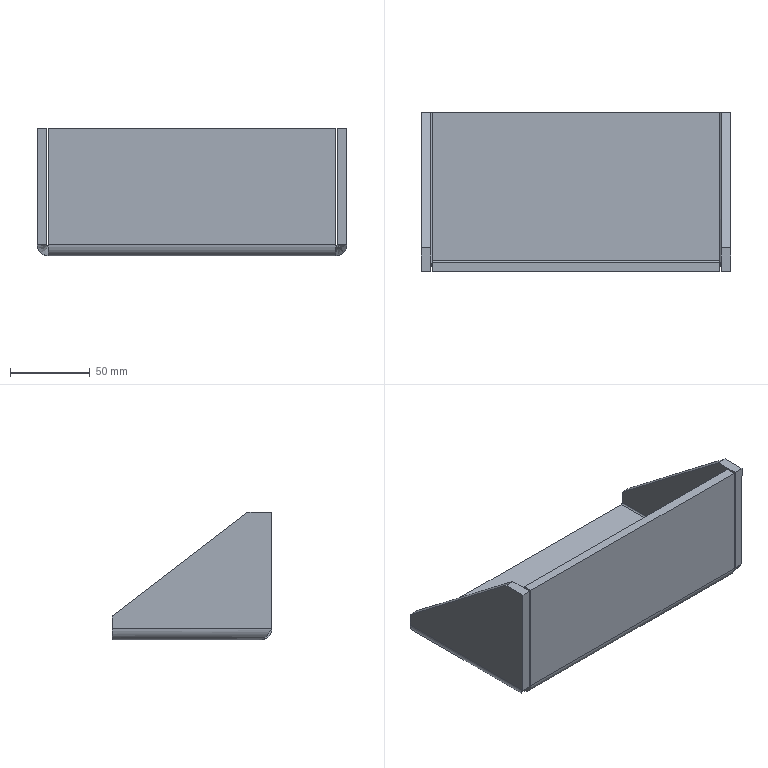Part | SolidWorks | features Chamfer 2, CornerFeat 2, EdgeFlange 2, FlatPattern 1, SMBaseFlange 1, SheetMetal 1 | 1 solid | 32 faces | box 194 x 100 x 80 mm | volume 247792 mm3 | plane 24 | cylinder 6 | spline 2 | commonest cylinder face diameters 2 x3 14 x3
STEP:
#1=CARTESIAN_POINT('',(-90.,1.,-40.));
#2=VERTEX_POINT('',#1);
#3=CARTESIAN_POINT('',(90.,1.,-40.));
#4=VERTEX_POINT('',#3);
#5=CARTESIAN_POINT('',(90.,1.,-40.));
#6=DIRECTION('',(1.,0.,0.));
#7=VECTOR('',#6,1000.);
#8=LINE('',#5,#7);
#9=EDGE_CURVE('',#2,#4,#8,.T.);
#10=ORIENTED_EDGE('',*,*,#9,.F.);
#11=CARTESIAN_POINT('',(-90.,94.,-40.));
#12=VERTEX_POINT('',#11);
#13=CARTESIAN_POINT('',(-90.,0.,-40.));
#14=DIRECTION('',(0.,1.,0.));
#15=VECTOR('',#14,1000.);
#16=LINE('',#13,#15);
#17=EDGE_CURVE('',#2,#12,#16,.T.);
#18=ORIENTED_EDGE('',*,*,#17,.T.);
#19=CARTESIAN_POINT('',(90.,94.,-40.));
#20=VERTEX_POINT('',#19);
#21=CARTESIAN_POINT('',(0.,94.,-40.));
#22=DIRECTION('',(1.,0.,0.));
#23=VECTOR('',#22,1000.);
#24=LINE('',#21,#23);
#25=EDGE_CURVE('',#12,#20,#24,.T.);
#26=ORIENTED_EDGE('',*,*,#25,.T.);
#27=CARTESIAN_POINT('',(90.,0.,-40.));
#28=DIRECTION('',(0.,-1.,0.));
#29=VECTOR('',#28,1000.);
#30=LINE('',#27,#29);
#31=EDGE_CURVE('',#20,#4,#30,.T.);
#32=ORIENTED_EDGE('',*,*,#31,.T.);
#33=EDGE_LOOP('',(#10,#18,#26,#32));
#34=FACE_OUTER_BOUND('',#33,.T.);
#35=CARTESIAN_POINT('',(0.,0.,-40.));
#36=DIRECTION('',(0.,0.,1.));
#37=DIRECTION('',(0.,-1.,0.));
#38=AXIS2_PLACEMENT_3D('',#35,#36,#37);
#39=PLANE('',#38);
#40=ADVANCED_FACE('',(#34),#39,.F.);
#41=CARTESIAN_POINT('',(-90.,1.,-34.));
#42=VERTEX_POINT('',#41);
#43=CARTESIAN_POINT('',(-90.,94.,-34.));
#44=VERTEX_POINT('',#43);
#45=CARTESIAN_POINT('',(-90.,94.,-34.));
#46=DIRECTION('',(0.,1.,0.));
#47=VECTOR('',#46,1000.);
#48=LINE('',#45,#47);
#49=EDGE_CURVE('',#42,#44,#48,.T.);
#50=ORIENTED_EDGE('',*,*,#49,.F.);
#51=CARTESIAN_POINT('',(90.,1.,-34.));
#52=VERTEX_POINT('',#51);
#53=CARTESIAN_POINT('',(90.,1.,-34.));
#54=DIRECTION('',(-1.,0.,0.));
#55=VECTOR('',#54,1000.);
#56=LINE('',#53,#55);
#57=EDGE_CURVE('',#52,#42,#56,.T.);
#58=ORIENTED_EDGE('',*,*,#57,.F.);
#59=CARTESIAN_POINT('',(90.,94.,-34.));
#60=VERTEX_POINT('',#59);
#61=CARTESIAN_POINT('',(90.,0.,-34.));
#62=DIRECTION('',(0.,-1.,0.));
#63=VECTOR('',#62,1000.);
#64=LINE('',#61,#63);
#65=EDGE_CURVE('',#60,#52,#64,.T.);
#66=ORIENTED_EDGE('',*,*,#65,.F.);
#67=CARTESIAN_POINT('',(90.,94.,-34.));
#68=DIRECTION('',(1.,0.,0.));
#69=VECTOR('',#68,1000.);
#70=LINE('',#67,#69);
#71=EDGE_CURVE('',#44,#60,#70,.T.);
#72=ORIENTED_EDGE('',*,*,#71,.F.);
#73=EDGE_LOOP('',(#50,#58,#66,#72));
#74=FACE_OUTER_BOUND('',#73,.T.);
#75=CARTESIAN_POINT('',(0.,0.,-34.));
#76=DIRECTION('',(0.,0.,1.));
#77=DIRECTION('',(0.,-1.,0.));
#78=AXIS2_PLACEMENT_3D('',#75,#76,#77);
#79=PLANE('',#78);
#80=ADVANCED_FACE('',(#74),#79,.T.);
#81=ORIENTED_EDGE('',*,*,#71,.T.);
#82=CARTESIAN_POINT('',(90.,94.,-40.));
#83=DIRECTION('',(0.,0.,1.));
#84=VECTOR('',#83,1000.);
#85=LINE('',#82,#84);
#86=EDGE_CURVE('',#20,#60,#85,.T.);
#87=ORIENTED_EDGE('',*,*,#86,.F.);
#88=ORIENTED_EDGE('',*,*,#25,.F.);
#89=CARTESIAN_POINT('',(-90.,94.,-40.));
#90=DIRECTION('',(0.,0.,1.));
#91=VECTOR('',#90,1000.);
#92=LINE('',#89,#91);
#93=EDGE_CURVE('',#12,#44,#92,.T.);
#94=ORIENTED_EDGE('',*,*,#93,.T.);
#95=EDGE_LOOP('',(#81,#87,#88,#94));
#96=FACE_OUTER_BOUND('',#95,.T.);
#97=CARTESIAN_POINT('',(90.,94.,-40.));
#98=DIRECTION('',(0.,-1.,0.));
#99=DIRECTION('',(0.,0.,-1.));
#100=AXIS2_PLACEMENT_3D('',#97,#98,#99);
#101=PLANE('',#100);
#102=ADVANCED_FACE('',(#96),#101,.F.);
#103=CARTESIAN_POINT('',(-97.,9.,40.));
#104=VERTEX_POINT('',#103);
#105=CARTESIAN_POINT('',(-97.,94.,-25.));
#106=VERTEX_POINT('',#105);
#107=CARTESIAN_POINT('',(-97.,94.,-25.));
#108=DIRECTION('',(0.,0.7944,-0.6075));
#109=VECTOR('',#108,1000.);
#110=LINE('',#107,#109);
#111=EDGE_CURVE('',#104,#106,#110,.T.);
#112=ORIENTED_EDGE('',*,*,#111,.F.);
#113=CARTESIAN_POINT('',(-91.,9.,40.));
#114=VERTEX_POINT('',#113);
#115=CARTESIAN_POINT('',(-97.,9.,40.));
#116=DIRECTION('',(-1.,0.,0.));
#117=VECTOR('',#116,1000.);
#118=LINE('',#115,#117);
#119=EDGE_CURVE('',#114,#104,#118,.T.);
#120=ORIENTED_EDGE('',*,*,#119,.F.);
#121=CARTESIAN_POINT('',(-91.,94.,-25.));
#122=VERTEX_POINT('',#121);
#123=CARTESIAN_POINT('',(-91.,22.622,29.583));
#124=DIRECTION('',(0.,-0.7944,0.6075));
#125=VECTOR('',#124,1000.);
#126=LINE('',#123,#125);
#127=EDGE_CURVE('',#122,#114,#126,.T.);
#128=ORIENTED_EDGE('',*,*,#127,.F.);
#129=CARTESIAN_POINT('',(-97.,94.,-25.));
#130=DIRECTION('',(1.,0.,0.));
#131=VECTOR('',#130,1000.);
#132=LINE('',#129,#131);
#133=EDGE_CURVE('',#106,#122,#132,.T.);
#134=ORIENTED_EDGE('',*,*,#133,.F.);
#135=EDGE_LOOP('',(#112,#120,#128,#134));
#136=FACE_OUTER_BOUND('',#135,.T.);
#137=CARTESIAN_POINT('',(-97.,94.,-25.));
#138=DIRECTION('',(0.,-0.6075,-0.7944));
#139=DIRECTION('',(1.,0.,0.));
#140=AXIS2_PLACEMENT_3D('',#137,#138,#139);
#141=PLANE('',#140);
#142=ADVANCED_FACE('',(#136),#141,.F.);
#143=CARTESIAN_POINT('',(-91.,-6.,40.));
#144=VERTEX_POINT('',#143);
#145=CARTESIAN_POINT('',(-91.,94.,40.));
#146=DIRECTION('',(0.,1.,0.));
#147=VECTOR('',#146,1000.);
#148=LINE('',#145,#147);
#149=EDGE_CURVE('',#144,#114,#148,.T.);
#150=ORIENTED_EDGE('',*,*,#149,.T.);
#151=ORIENTED_EDGE('',*,*,#119,.T.);
#152=CARTESIAN_POINT('',(-97.,-6.,40.));
#153=VERTEX_POINT('',#152);
#154=CARTESIAN_POINT('',(-97.,0.,40.));
#155=DIRECTION('',(0.,1.,0.));
#156=VECTOR('',#155,1000.);
#157=LINE('',#154,#156);
#158=EDGE_CURVE('',#153,#104,#157,.T.);
#159=ORIENTED_EDGE('',*,*,#158,.F.);
#160=CARTESIAN_POINT('',(-97.,-6.,40.));
#161=DIRECTION('',(1.,0.,0.));
#162=VECTOR('',#161,1000.);
#163=LINE('',#160,#162);
#164=EDGE_CURVE('',#153,#144,#163,.T.);
#165=ORIENTED_EDGE('',*,*,#164,.T.);
#166=EDGE_LOOP('',(#150,#151,#159,#165));
#167=FACE_OUTER_BOUND('',#166,.T.);
#168=CARTESIAN_POINT('',(-97.,94.,40.));
#169=DIRECTION('',(0.,0.,-1.));
#170=DIRECTION('',(-1.,0.,0.));
#171=AXIS2_PLACEMENT_3D('',#168,#169,#170);
#172=PLANE('',#171);
#173=ADVANCED_FACE('',(#167),#172,.F.);
#174=ORIENTED_EDGE('',*,*,#158,.T.);
#175=ORIENTED_EDGE('',*,*,#111,.T.);
#176=CARTESIAN_POINT('',(-97.,94.,-33.));
#177=VERTEX_POINT('',#176);
#178=CARTESIAN_POINT('',(-97.,94.,0.));
#179=DIRECTION('',(0.,0.,-1.));
#180=VECTOR('',#179,1000.);
#181=LINE('',#178,#180);
#182=EDGE_CURVE('',#106,#177,#181,.T.);
#183=ORIENTED_EDGE('',*,*,#182,.T.);
#184=CARTESIAN_POINT('',(-97.,-6.,-33.));
#185=VERTEX_POINT('',#184);
#186=CARTESIAN_POINT('',(-97.,94.,-33.));
#187=DIRECTION('',(0.,1.,0.));
#188=VECTOR('',#187,1000.);
#189=LINE('',#186,#188);
#190=EDGE_CURVE('',#185,#177,#189,.T.);
#191=ORIENTED_EDGE('',*,*,#190,.F.);
#192=CARTESIAN_POINT('',(-97.,-6.,-33.));
#193=DIRECTION('',(0.,0.,1.));
#194=VECTOR('',#193,1000.);
#195=LINE('',#192,#194);
#196=EDGE_CURVE('',#185,#153,#195,.T.);
#197=ORIENTED_EDGE('',*,*,#196,.T.);
#198=EDGE_LOOP('',(#174,#175,#183,#191,#197));
#199=FACE_OUTER_BOUND('',#198,.T.);
#200=CARTESIAN_POINT('',(-97.,0.,0.));
#201=DIRECTION('',(1.,0.,0.));
#202=DIRECTION('',(0.,0.,-1.));
#203=AXIS2_PLACEMENT_3D('',#200,#201,#202);
#204=PLANE('',#203);
#205=ADVANCED_FACE('',(#199),#204,.F.);
#206=CARTESIAN_POINT('',(-91.,-6.,-33.));
#207=VERTEX_POINT('',#206);
#208=CARTESIAN_POINT('',(-91.,-6.,-33.));
#209=DIRECTION('',(0.,0.,1.));
#210=VECTOR('',#209,1000.);
#211=LINE('',#208,#210);
#212=EDGE_CURVE('',#207,#144,#211,.T.);
#213=ORIENTED_EDGE('',*,*,#212,.T.);
#214=ORIENTED_EDGE('',*,*,#164,.F.);
#215=ORIENTED_EDGE('',*,*,#196,.F.);
#216=CARTESIAN_POINT('',(-97.,-6.,-33.));
#217=CARTESIAN_POINT('',(-95.,-6.,-33.));
#218=CARTESIAN_POINT('',(-93.,-6.,-33.));
#219=CARTESIAN_POINT('',(-91.,-6.,-33.));
#220=B_SPLINE_CURVE_WITH_KNOTS('',3,(#216,#217,#218,#219),.UNSPECIFIED.,.F.,.F.,(4,4),(0.,1.),.UNSPECIFIED.);
#221=EDGE_CURVE('',#185,#207,#220,.T.);
#222=ORIENTED_EDGE('',*,*,#221,.T.);
#223=EDGE_LOOP('',(#213,#214,#215,#222));
#224=FACE_OUTER_BOUND('',#223,.T.);
#225=CARTESIAN_POINT('',(-97.,-6.,-33.));
#226=DIRECTION('',(0.,1.,0.));
#227=DIRECTION('',(-1.,0.,0.));
#228=AXIS2_PLACEMENT_3D('',#225,#226,#227);
#229=PLANE('',#228);
#230=ADVANCED_FACE('',(#224),#229,.F.);
#231=CARTESIAN_POINT('',(-91.,94.,-33.));
#232=VERTEX_POINT('',#231);
#233=CARTESIAN_POINT('',(-91.,94.,-34.));
#234=DIRECTION('',(0.,0.,-1.));
#235=VECTOR('',#234,1000.);
#236=LINE('',#233,#235);
#237=EDGE_CURVE('',#122,#232,#236,.T.);
#238=ORIENTED_EDGE('',*,*,#237,.F.);
#239=ORIENTED_EDGE('',*,*,#127,.T.);
#240=ORIENTED_EDGE('',*,*,#149,.F.);
#241=ORIENTED_EDGE('',*,*,#212,.F.);
#242=CARTESIAN_POINT('',(-91.,94.,-33.));
#243=DIRECTION('',(0.,-1.,0.));
#244=VECTOR('',#243,1000.);
#245=LINE('',#242,#244);
#246=EDGE_CURVE('',#232,#207,#245,.T.);
#247=ORIENTED_EDGE('',*,*,#246,.F.);
#248=EDGE_LOOP('',(#238,#239,#240,#241,#247));
#249=FACE_OUTER_BOUND('',#248,.T.);
#250=CARTESIAN_POINT('',(-91.,0.,0.));
#251=DIRECTION('',(1.,0.,0.));
#252=DIRECTION('',(0.,0.,-1.));
#253=AXIS2_PLACEMENT_3D('',#250,#251,#252);
#254=PLANE('',#253);
#255=ADVANCED_FACE('',(#249),#254,.T.);
#256=ORIENTED_EDGE('',*,*,#182,.F.);
#257=ORIENTED_EDGE('',*,*,#133,.T.);
#258=ORIENTED_EDGE('',*,*,#237,.T.);
#259=CARTESIAN_POINT('',(-97.,94.,-33.));
#260=DIRECTION('',(-1.,0.,0.));
#261=VECTOR('',#260,1000.);
#262=LINE('',#259,#261);
#263=EDGE_CURVE('',#232,#177,#262,.T.);
#264=ORIENTED_EDGE('',*,*,#263,.T.);
#265=EDGE_LOOP('',(#256,#257,#258,#264));
#266=FACE_OUTER_BOUND('',#265,.T.);
#267=CARTESIAN_POINT('',(-97.,94.,-34.));
#268=DIRECTION('',(0.,-1.,0.));
#269=DIRECTION('',(0.,0.,-1.));
#270=AXIS2_PLACEMENT_3D('',#267,#268,#269);
#271=PLANE('',#270);
#272=ADVANCED_FACE('',(#266),#271,.F.);
#273=ORIENTED_EDGE('',*,*,#263,.F.);
#274=CARTESIAN_POINT('',(-90.,94.,-33.));
#275=DIRECTION('',(0.,-1.,0.));
#276=DIRECTION('',(0.,0.,-1.));
#277=AXIS2_PLACEMENT_3D('',#274,#275,#276);
#278=CIRCLE('',#277,1.);
#279=EDGE_CURVE('',#232,#44,#278,.T.);
#280=ORIENTED_EDGE('',*,*,#279,.T.);
#281=ORIENTED_EDGE('',*,*,#93,.F.);
#282=CARTESIAN_POINT('',(-90.,94.,-33.));
#283=DIRECTION('',(0.,-1.,0.));
#284=DIRECTION('',(0.,0.,-1.));
#285=AXIS2_PLACEMENT_3D('',#282,#283,#284);
#286=CIRCLE('',#285,7.);
#287=EDGE_CURVE('',#177,#12,#286,.T.);
#288=ORIENTED_EDGE('',*,*,#287,.F.);
#289=EDGE_LOOP('',(#273,#280,#281,#288));
#290=FACE_OUTER_BOUND('',#289,.T.);
#291=CARTESIAN_POINT('',(-90.,94.,-33.));
#292=DIRECTION('',(0.,1.,0.));
#293=DIRECTION('',(0.,0.,1.));
#294=AXIS2_PLACEMENT_3D('',#291,#292,#293);
#295=PLANE('',#294);
#296=ADVANCED_FACE('',(#290),#295,.T.);
#297=CARTESIAN_POINT('',(-90.,1.,-34.));
#298=CARTESIAN_POINT('',(-90.131,0.4159,-34.));
#299=CARTESIAN_POINT('',(-90.262,-0.1669,-33.974));
#300=CARTESIAN_POINT('',(-90.504,-1.335,-33.874));
#301=CARTESIAN_POINT('',(-90.615,-1.918,-33.799));
#302=CARTESIAN_POINT('',(-90.8,-3.085,-33.614));
#303=CARTESIAN_POINT('',(-90.874,-3.669,-33.503));
#304=CARTESIAN_POINT('',(-90.974,-4.834,-33.262));
#305=CARTESIAN_POINT('',(-91.,-5.416,-33.131));
#306=CARTESIAN_POINT('',(-91.,-6.,-33.));
#307=B_SPLINE_CURVE_WITH_KNOTS('',3,(#297,#298,#299,#300,#301,#302,#303,#304,#305,#306),.UNSPECIFIED.,.F.,.F.,(4,2,2,2,4),(0.,0.001794,0.003587,0.005381,0.007175),.UNSPECIFIED.);
#308=EDGE_CURVE('',#42,#207,#307,.T.);
#309=ORIENTED_EDGE('',*,*,#308,.T.);
#310=ORIENTED_EDGE('',*,*,#221,.F.);
#311=CARTESIAN_POINT('',(-90.,1.,-40.));
#312=CARTESIAN_POINT('',(-90.462,0.7056,-40.));
#313=CARTESIAN_POINT('',(-90.919,0.4151,-39.954));
#314=CARTESIAN_POINT('',(-91.814,-0.1663,-39.776));
#315=CARTESIAN_POINT('',(-92.256,-0.4585,-39.643));
#316=CARTESIAN_POINT('',(-93.108,-1.046,-39.289));
#317=CARTESIAN_POINT('',(-93.511,-1.336,-39.073));
#318=CARTESIAN_POINT('',(-94.269,-1.916,-38.566));
#319=CARTESIAN_POINT('',(-94.625,-2.207,-38.275));
#320=CARTESIAN_POINT('',(-95.604,-3.089,-37.295));
#321=CARTESIAN_POINT('',(-96.114,-3.662,-36.532));
#322=CARTESIAN_POINT('',(-96.821,-4.839,-34.824));
#323=CARTESIAN_POINT('',(-97.,-5.411,-33.925));
#324=CARTESIAN_POINT('',(-97.,-6.,-33.));
#325=B_SPLINE_CURVE_WITH_KNOTS('',3,(#311,#312,#313,#314,#315,#316,#317,#318,#319,#320,#321,#322,#323,#324),.UNSPECIFIED.,.F.,.F.,(4,2,2,2,2,2,4),(0.,0.001624,0.003248,0.004872,0.006496,0.009744,0.01299),.UNSPECIFIED.);
#326=EDGE_CURVE('',#2,#185,#325,.T.);
#327=ORIENTED_EDGE('',*,*,#326,.F.);
#328=CARTESIAN_POINT('',(-90.,1.,-34.));
#329=CARTESIAN_POINT('',(-90.,1.,-36.));
#330=CARTESIAN_POINT('',(-90.,1.,-38.));
#331=CARTESIAN_POINT('',(-90.,1.,-40.));
#332=B_SPLINE_CURVE_WITH_KNOTS('',3,(#328,#329,#330,#331),.UNSPECIFIED.,.F.,.F.,(4,4),(0.,1.),.UNSPECIFIED.);
#333=EDGE_CURVE('',#42,#2,#332,.T.);
#334=ORIENTED_EDGE('',*,*,#333,.F.);
#335=EDGE_LOOP('',(#309,#310,#327,#334));
#336=FACE_OUTER_BOUND('',#335,.T.);
#337=CARTESIAN_POINT('',(-90.,1.,-40.061));
#338=CARTESIAN_POINT('',(-90.924,0.4166,-40.061));
#339=CARTESIAN_POINT('',(-91.848,-0.1667,-39.877));
#340=CARTESIAN_POINT('',(-93.556,-1.333,-39.169));
#341=CARTESIAN_POINT('',(-94.339,-1.917,-38.646));
#342=CARTESIAN_POINT('',(-95.646,-3.083,-37.339));
#343=CARTESIAN_POINT('',(-96.169,-3.667,-36.556));
#344=CARTESIAN_POINT('',(-96.877,-4.833,-34.848));
#345=CARTESIAN_POINT('',(-97.061,-5.417,-33.924));
#346=CARTESIAN_POINT('',(-97.061,-6.,-33.));
#347=CARTESIAN_POINT('',(-90.,1.,-40.));
#348=CARTESIAN_POINT('',(-90.916,0.4166,-40.));
#349=CARTESIAN_POINT('',(-91.832,-0.1667,-39.818));
#350=CARTESIAN_POINT('',(-93.525,-1.333,-39.117));
#351=CARTESIAN_POINT('',(-94.302,-1.917,-38.598));
#352=CARTESIAN_POINT('',(-95.598,-3.083,-37.302));
#353=CARTESIAN_POINT('',(-96.117,-3.667,-36.525));
#354=CARTESIAN_POINT('',(-96.818,-4.833,-34.832));
#355=CARTESIAN_POINT('',(-97.,-5.417,-33.916));
#356=CARTESIAN_POINT('',(-97.,-6.,-33.));
#357=CARTESIAN_POINT('',(-90.,1.,-34.));
#358=CARTESIAN_POINT('',(-90.131,0.4167,-34.));
#359=CARTESIAN_POINT('',(-90.262,-0.1667,-33.974));
#360=CARTESIAN_POINT('',(-90.504,-1.333,-33.874));
#361=CARTESIAN_POINT('',(-90.615,-1.917,-33.8));
#362=CARTESIAN_POINT('',(-90.8,-3.083,-33.615));
#363=CARTESIAN_POINT('',(-90.874,-3.667,-33.504));
#364=CARTESIAN_POINT('',(-90.974,-4.833,-33.262));
#365=CARTESIAN_POINT('',(-91.,-5.417,-33.131));
#366=CARTESIAN_POINT('',(-91.,-6.,-33.));
#367=CARTESIAN_POINT('',(-90.,1.,-33.94));
#368=CARTESIAN_POINT('',(-90.123,0.4167,-33.94));
#369=CARTESIAN_POINT('',(-90.246,-0.1667,-33.916));
#370=CARTESIAN_POINT('',(-90.473,-1.333,-33.821));
#371=CARTESIAN_POINT('',(-90.578,-1.917,-33.752));
#372=CARTESIAN_POINT('',(-90.752,-3.083,-33.578));
#373=CARTESIAN_POINT('',(-90.821,-3.667,-33.473));
#374=CARTESIAN_POINT('',(-90.916,-4.833,-33.246));
#375=CARTESIAN_POINT('',(-90.94,-5.417,-33.123));
#376=CARTESIAN_POINT('',(-90.94,-6.,-33.));
#377=B_SPLINE_SURFACE_WITH_KNOTS('',1,3,((#337,#338,#339,#340,#341,#342,#343,#344,#345,#346),(#347,#348,#349,#350,#351,#352,#353,#354,#355,#356),(#357,#358,#359,#360,#361,#362,#363,#364,#365,#366),(#367,#368,#369,#370,#371,#372,#373,#374,#375,#376)),.UNSPECIFIED.,.F.,.F.,.F.,(2,1,1,2),(4,2,2,2,4),(-0.0101,0.,1.,1.01),(0.,0.25,0.5,0.75,1.),.UNSPECIFIED.);
#378=ADVANCED_FACE('',(#336),#377,.T.);
#379=ORIENTED_EDGE('',*,*,#17,.F.);
#380=ORIENTED_EDGE('',*,*,#326,.T.);
#381=ORIENTED_EDGE('',*,*,#190,.T.);
#382=ORIENTED_EDGE('',*,*,#287,.T.);
#383=EDGE_LOOP('',(#379,#380,#381,#382));
#384=FACE_OUTER_BOUND('',#383,.T.);
#385=CARTESIAN_POINT('',(-90.,144.377,-33.));
#386=DIRECTION('',(0.,-1.,0.));
#387=DIRECTION('',(0.,0.,-1.));
#388=AXIS2_PLACEMENT_3D('',#385,#386,#387);
#389=CYLINDRICAL_SURFACE('',#388,7.);
#390=ADVANCED_FACE('',(#384),#389,.T.);
#391=ORIENTED_EDGE('',*,*,#49,.T.);
#392=ORIENTED_EDGE('',*,*,#279,.F.);
#393=ORIENTED_EDGE('',*,*,#246,.T.);
#394=ORIENTED_EDGE('',*,*,#308,.F.);
#395=EDGE_LOOP('',(#391,#392,#393,#394));
#396=FACE_OUTER_BOUND('',#395,.T.);
#397=CARTESIAN_POINT('',(-90.,144.377,-33.));
#398=DIRECTION('',(0.,-1.,0.));
#399=DIRECTION('',(0.,0.,-1.));
#400=AXIS2_PLACEMENT_3D('',#397,#398,#399);
#401=CYLINDRICAL_SURFACE('',#400,1.);
#402=ADVANCED_FACE('',(#396),#401,.F.);
#403=CARTESIAN_POINT('',(97.,9.,40.));
#404=VERTEX_POINT('',#403);
#405=CARTESIAN_POINT('',(97.,-6.,40.));
#406=VERTEX_POINT('',#405);
#407=CARTESIAN_POINT('',(97.,0.,40.));
#408=DIRECTION('',(0.,-1.,0.));
#409=VECTOR('',#408,1000.);
#410=LINE('',#407,#409);
#411=EDGE_CURVE('',#404,#406,#410,.T.);
#412=ORIENTED_EDGE('',*,*,#411,.F.);
#413=CARTESIAN_POINT('',(91.,9.,40.));
#414=VERTEX_POINT('',#413);
#415=CARTESIAN_POINT('',(97.,9.,40.));
#416=DIRECTION('',(-1.,0.,0.));
#417=VECTOR('',#416,1000.);
#418=LINE('',#415,#417);
#419=EDGE_CURVE('',#404,#414,#418,.T.);
#420=ORIENTED_EDGE('',*,*,#419,.T.);
#421=CARTESIAN_POINT('',(91.,-6.,40.));
#422=VERTEX_POINT('',#421);
#423=CARTESIAN_POINT('',(91.,1.,40.));
#424=DIRECTION('',(0.,-1.,0.));
#425=VECTOR('',#424,1000.);
#426=LINE('',#423,#425);
#427=EDGE_CURVE('',#414,#422,#426,.T.);
#428=ORIENTED_EDGE('',*,*,#427,.T.);
#429=CARTESIAN_POINT('',(97.,-6.,40.));
#430=DIRECTION('',(-1.,0.,0.));
#431=VECTOR('',#430,1000.);
#432=LINE('',#429,#431);
#433=EDGE_CURVE('',#406,#422,#432,.T.);
#434=ORIENTED_EDGE('',*,*,#433,.F.);
#435=EDGE_LOOP('',(#412,#420,#428,#434));
#436=FACE_OUTER_BOUND('',#435,.T.);
#437=CARTESIAN_POINT('',(97.,1.,40.));
#438=DIRECTION('',(0.,0.,-1.));
#439=DIRECTION('',(-1.,0.,0.));
#440=AXIS2_PLACEMENT_3D('',#437,#438,#439);
#441=PLANE('',#440);
#442=ADVANCED_FACE('',(#436),#441,.F.);
#443=CARTESIAN_POINT('',(97.,94.,-25.));
#444=VERTEX_POINT('',#443);
#445=CARTESIAN_POINT('',(97.,9.,40.));
#446=DIRECTION('',(0.,-0.7944,0.6075));
#447=VECTOR('',#446,1000.);
#448=LINE('',#445,#447);
#449=EDGE_CURVE('',#444,#404,#448,.T.);
#450=ORIENTED_EDGE('',*,*,#449,.F.);
#451=CARTESIAN_POINT('',(91.,94.,-25.));
#452=VERTEX_POINT('',#451);
#453=CARTESIAN_POINT('',(97.,94.,-25.));
#454=DIRECTION('',(1.,0.,0.));
#455=VECTOR('',#454,1000.);
#456=LINE('',#453,#455);
#457=EDGE_CURVE('',#452,#444,#456,.T.);
#458=ORIENTED_EDGE('',*,*,#457,.F.);
#459=CARTESIAN_POINT('',(91.,22.622,29.583));
#460=DIRECTION('',(0.,0.7944,-0.6075));
#461=VECTOR('',#460,1000.);
#462=LINE('',#459,#461);
#463=EDGE_CURVE('',#414,#452,#462,.T.);
#464=ORIENTED_EDGE('',*,*,#463,.F.);
#465=ORIENTED_EDGE('',*,*,#419,.F.);
#466=EDGE_LOOP('',(#450,#458,#464,#465));
#467=FACE_OUTER_BOUND('',#466,.T.);
#468=CARTESIAN_POINT('',(97.,9.,40.));
#469=DIRECTION('',(0.,-0.6075,-0.7944));
#470=DIRECTION('',(-1.,0.,0.));
#471=AXIS2_PLACEMENT_3D('',#468,#469,#470);
#472=PLANE('',#471);
#473=ADVANCED_FACE('',(#467),#472,.F.);
#474=CARTESIAN_POINT('',(97.,94.,-33.));
#475=VERTEX_POINT('',#474);
#476=CARTESIAN_POINT('',(97.,94.,0.));
#477=DIRECTION('',(0.,0.,1.));
#478=VECTOR('',#477,1000.);
#479=LINE('',#476,#478);
#480=EDGE_CURVE('',#475,#444,#479,.T.);
#481=ORIENTED_EDGE('',*,*,#480,.T.);
#482=ORIENTED_EDGE('',*,*,#449,.T.);
#483=ORIENTED_EDGE('',*,*,#411,.T.);
#484=CARTESIAN_POINT('',(97.,-6.,-33.));
#485=VERTEX_POINT('',#484);
#486=CARTESIAN_POINT('',(97.,-6.,-33.));
#487=DIRECTION('',(0.,0.,1.));
#488=VECTOR('',#487,1000.);
#489=LINE('',#486,#488);
#490=EDGE_CURVE('',#485,#406,#489,.T.);
#491=ORIENTED_EDGE('',*,*,#490,.F.);
#492=CARTESIAN_POINT('',(97.,1.,-33.));
#493=DIRECTION('',(0.,-1.,0.));
#494=VECTOR('',#493,1000.);
#495=LINE('',#492,#494);
#496=EDGE_CURVE('',#475,#485,#495,.T.);
#497=ORIENTED_EDGE('',*,*,#496,.F.);
#498=EDGE_LOOP('',(#481,#482,#483,#491,#497));
#499=FACE_OUTER_BOUND('',#498,.T.);
#500=CARTESIAN_POINT('',(97.,0.,0.));
#501=DIRECTION('',(-1.,0.,0.));
#502=DIRECTION('',(0.,0.,1.));
#503=AXIS2_PLACEMENT_3D('',#500,#501,#502);
#504=PLANE('',#503);
#505=ADVANCED_FACE('',(#499),#504,.F.);
#506=CARTESIAN_POINT('',(91.,94.,-33.));
#507=VERTEX_POINT('',#506);
#508=CARTESIAN_POINT('',(91.,94.,40.));
#509=DIRECTION('',(0.,0.,1.));
#510=VECTOR('',#509,1000.);
#511=LINE('',#508,#510);
#512=EDGE_CURVE('',#507,#452,#511,.T.);
#513=ORIENTED_EDGE('',*,*,#512,.T.);
#514=ORIENTED_EDGE('',*,*,#457,.T.);
#515=ORIENTED_EDGE('',*,*,#480,.F.);
#516=CARTESIAN_POINT('',(91.,94.,-33.));
#517=DIRECTION('',(1.,0.,0.));
#518=VECTOR('',#517,1000.);
#519=LINE('',#516,#518);
#520=EDGE_CURVE('',#507,#475,#519,.T.);
#521=ORIENTED_EDGE('',*,*,#520,.F.);
#522=EDGE_LOOP('',(#513,#514,#515,#521));
#523=FACE_OUTER_BOUND('',#522,.T.);
#524=CARTESIAN_POINT('',(97.,94.,40.));
#525=DIRECTION('',(0.,-1.,0.));
#526=DIRECTION('',(0.,0.,-1.));
#527=AXIS2_PLACEMENT_3D('',#524,#525,#526);
#528=PLANE('',#527);
#529=ADVANCED_FACE('',(#523),#528,.F.);
#530=ORIENTED_EDGE('',*,*,#427,.F.);
#531=ORIENTED_EDGE('',*,*,#463,.T.);
#532=ORIENTED_EDGE('',*,*,#512,.F.);
#533=CARTESIAN_POINT('',(91.,-6.,-33.));
#534=VERTEX_POINT('',#533);
#535=CARTESIAN_POINT('',(91.,1.,-33.));
#536=DIRECTION('',(0.,1.,0.));
#537=VECTOR('',#536,1000.);
#538=LINE('',#535,#537);
#539=EDGE_CURVE('',#534,#507,#538,.T.);
#540=ORIENTED_EDGE('',*,*,#539,.F.);
#541=CARTESIAN_POINT('',(91.,-6.,-33.));
#542=DIRECTION('',(0.,0.,1.));
#543=VECTOR('',#542,1000.);
#544=LINE('',#541,#543);
#545=EDGE_CURVE('',#534,#422,#544,.T.);
#546=ORIENTED_EDGE('',*,*,#545,.T.);
#547=EDGE_LOOP('',(#530,#531,#532,#540,#546));
#548=FACE_OUTER_BOUND('',#547,.T.);
#549=CARTESIAN_POINT('',(91.,0.,0.));
#550=DIRECTION('',(-1.,0.,0.));
#551=DIRECTION('',(0.,0.,1.));
#552=AXIS2_PLACEMENT_3D('',#549,#550,#551);
#553=PLANE('',#552);
#554=ADVANCED_FACE('',(#548),#553,.T.);
#555=ORIENTED_EDGE('',*,*,#545,.F.);
#556=CARTESIAN_POINT('',(97.,-6.,-33.));
#557=CARTESIAN_POINT('',(91.,-6.,-33.));
#558=B_SPLINE_CURVE_WITH_KNOTS('',1,(#556,#557),.UNSPECIFIED.,.F.,.F.,(2,2),(0.,1.),.UNSPECIFIED.);
#559=EDGE_CURVE('',#485,#534,#558,.T.);
#560=ORIENTED_EDGE('',*,*,#559,.F.);
#561=ORIENTED_EDGE('',*,*,#490,.T.);
#562=ORIENTED_EDGE('',*,*,#433,.T.);
#563=EDGE_LOOP('',(#555,#560,#561,#562));
#564=FACE_OUTER_BOUND('',#563,.T.);
#565=CARTESIAN_POINT('',(97.,-6.,-33.));
#566=DIRECTION('',(0.,-1.,0.));
#567=DIRECTION('',(1.,0.,0.));
#568=AXIS2_PLACEMENT_3D('',#565,#566,#567);
#569=PLANE('',#568);
#570=ADVANCED_FACE('',(#564),#569,.T.);
#571=ORIENTED_EDGE('',*,*,#559,.T.);
#572=CARTESIAN_POINT('',(91.,-6.,-33.));
#573=CARTESIAN_POINT('',(91.,-5.416,-33.131));
#574=CARTESIAN_POINT('',(90.974,-4.833,-33.262));
#575=CARTESIAN_POINT('',(90.874,-3.665,-33.504));
#576=CARTESIAN_POINT('',(90.799,-3.082,-33.615));
#577=CARTESIAN_POINT('',(90.614,-1.915,-33.8));
#578=CARTESIAN_POINT('',(90.503,-1.331,-33.874));
#579=CARTESIAN_POINT('',(90.262,-0.1663,-33.974));
#580=CARTESIAN_POINT('',(90.131,0.4159,-34.));
#581=CARTESIAN_POINT('',(90.,1.,-34.));
#582=B_SPLINE_CURVE_WITH_KNOTS('',3,(#572,#573,#574,#575,#576,#577,#578,#579,#580,#581),.UNSPECIFIED.,.F.,.F.,(4,2,2,2,4),(0.,0.001794,0.003587,0.005381,0.007175),.UNSPECIFIED.);
#583=EDGE_CURVE('',#534,#52,#582,.T.);
#584=ORIENTED_EDGE('',*,*,#583,.T.);
#585=CARTESIAN_POINT('',(90.,1.,-34.));
#586=CARTESIAN_POINT('',(90.,1.,-40.));
#587=B_SPLINE_CURVE_WITH_KNOTS('',1,(#585,#586),.UNSPECIFIED.,.F.,.F.,(2,2),(0.,1.),.UNSPECIFIED.);
#588=EDGE_CURVE('',#52,#4,#587,.T.);
#589=ORIENTED_EDGE('',*,*,#588,.T.);
#590=CARTESIAN_POINT('',(97.,-6.,-33.));
#591=CARTESIAN_POINT('',(97.,-5.706,-33.462));
#592=CARTESIAN_POINT('',(96.954,-5.415,-33.919));
#593=CARTESIAN_POINT('',(96.821,-4.979,-34.591));
#594=CARTESIAN_POINT('',(96.765,-4.833,-34.813));
#595=CARTESIAN_POINT('',(96.632,-4.541,-35.252));
#596=CARTESIAN_POINT('',(96.554,-4.394,-35.469));
#597=CARTESIAN_POINT('',(96.289,-3.954,-36.108));
#598=CARTESIAN_POINT('',(96.073,-3.664,-36.511));
#599=CARTESIAN_POINT('',(95.566,-3.084,-37.269));
#600=CARTESIAN_POINT('',(95.274,-2.792,-37.625));
#601=CARTESIAN_POINT('',(94.622,-2.205,-38.278));
#602=CARTESIAN_POINT('',(94.267,-1.915,-38.568));
#603=CARTESIAN_POINT('',(93.509,-1.334,-39.074));
#604=CARTESIAN_POINT('',(93.104,-1.043,-39.291));
#605=CARTESIAN_POINT('',(91.824,-0.1611,-39.821));
#606=CARTESIAN_POINT('',(90.925,0.4113,-40.));
#607=CARTESIAN_POINT('',(90.,1.,-40.));
#608=B_SPLINE_CURVE_WITH_KNOTS('',3,(#590,#591,#592,#593,#594,#595,#596,#597,#598,#599,#600,#601,#602,#603,#604,#605,#606,#607),.UNSPECIFIED.,.F.,.F.,(4,2,2,2,2,2,2,2,4),(0.,0.001624,0.002437,0.003249,0.004873,0.006498,0.008122,0.009746,0.013),.UNSPECIFIED.);
#609=EDGE_CURVE('',#485,#4,#608,.T.);
#610=ORIENTED_EDGE('',*,*,#609,.F.);
#611=EDGE_LOOP('',(#571,#584,#589,#610));
#612=FACE_OUTER_BOUND('',#611,.T.);
#613=CARTESIAN_POINT('',(97.06,-6.,-33.));
#614=CARTESIAN_POINT('',(97.06,-5.417,-33.924));
#615=CARTESIAN_POINT('',(96.876,-4.833,-34.848));
#616=CARTESIAN_POINT('',(96.169,-3.667,-36.556));
#617=CARTESIAN_POINT('',(95.646,-3.083,-37.339));
#618=CARTESIAN_POINT('',(94.339,-1.917,-38.646));
#619=CARTESIAN_POINT('',(93.556,-1.333,-39.169));
#620=CARTESIAN_POINT('',(91.848,-0.1667,-39.876));
#621=CARTESIAN_POINT('',(90.924,0.4166,-40.06));
#622=CARTESIAN_POINT('',(90.,1.,-40.06));
#623=CARTESIAN_POINT('',(97.,-6.,-33.));
#624=CARTESIAN_POINT('',(97.,-5.417,-33.916));
#625=CARTESIAN_POINT('',(96.818,-4.833,-34.832));
#626=CARTESIAN_POINT('',(96.117,-3.667,-36.525));
#627=CARTESIAN_POINT('',(95.598,-3.083,-37.302));
#628=CARTESIAN_POINT('',(94.302,-1.917,-38.598));
#629=CARTESIAN_POINT('',(93.525,-1.333,-39.117));
#630=CARTESIAN_POINT('',(91.832,-0.1667,-39.818));
#631=CARTESIAN_POINT('',(90.916,0.4166,-40.));
#632=CARTESIAN_POINT('',(90.,1.,-40.));
#633=CARTESIAN_POINT('',(91.,-6.,-33.));
#634=CARTESIAN_POINT('',(91.,-5.417,-33.131));
#635=CARTESIAN_POINT('',(90.974,-4.833,-33.262));
#636=CARTESIAN_POINT('',(90.874,-3.667,-33.504));
#637=CARTESIAN_POINT('',(90.8,-3.083,-33.615));
#638=CARTESIAN_POINT('',(90.615,-1.917,-33.8));
#639=CARTESIAN_POINT('',(90.504,-1.333,-33.874));
#640=CARTESIAN_POINT('',(90.262,-0.1667,-33.974));
#641=CARTESIAN_POINT('',(90.131,0.4167,-34.));
#642=CARTESIAN_POINT('',(90.,1.,-34.));
#643=CARTESIAN_POINT('',(90.939,-6.,-33.));
#644=CARTESIAN_POINT('',(90.939,-5.417,-33.123));
#645=CARTESIAN_POINT('',(90.915,-4.833,-33.246));
#646=CARTESIAN_POINT('',(90.821,-3.667,-33.473));
#647=CARTESIAN_POINT('',(90.751,-3.083,-33.577));
#648=CARTESIAN_POINT('',(90.577,-1.917,-33.751));
#649=CARTESIAN_POINT('',(90.473,-1.333,-33.821));
#650=CARTESIAN_POINT('',(90.246,-0.1667,-33.915));
#651=CARTESIAN_POINT('',(90.123,0.4167,-33.939));
#652=CARTESIAN_POINT('',(90.,1.,-33.939));
#653=B_SPLINE_SURFACE_WITH_KNOTS('',1,3,((#613,#614,#615,#616,#617,#618,#619,#620,#621,#622),(#623,#624,#625,#626,#627,#628,#629,#630,#631,#632),(#633,#634,#635,#636,#637,#638,#639,#640,#641,#642),(#643,#644,#645,#646,#647,#648,#649,#650,#651,#652)),.UNSPECIFIED.,.F.,.F.,.F.,(2,1,1,2),(4,2,2,2,4),(-0.01,0.,1.,1.01),(0.,0.25,0.5,0.75,1.),.UNSPECIFIED.);
#654=ADVANCED_FACE('',(#612),#653,.T.);
#655=CARTESIAN_POINT('',(90.,94.,-33.));
#656=DIRECTION('',(0.,-1.,0.));
#657=DIRECTION('',(0.,0.,1.));
#658=AXIS2_PLACEMENT_3D('',#655,#656,#657);
#659=CIRCLE('',#658,1.);
#660=EDGE_CURVE('',#60,#507,#659,.T.);
#661=ORIENTED_EDGE('',*,*,#660,.T.);
#662=ORIENTED_EDGE('',*,*,#520,.T.);
#663=CARTESIAN_POINT('',(90.,94.,-33.));
#664=DIRECTION('',(0.,-1.,0.));
#665=DIRECTION('',(0.,0.,-1.));
#666=AXIS2_PLACEMENT_3D('',#663,#664,#665);
#667=CIRCLE('',#666,7.);
#668=EDGE_CURVE('',#20,#475,#667,.T.);
#669=ORIENTED_EDGE('',*,*,#668,.F.);
#670=ORIENTED_EDGE('',*,*,#86,.T.);
#671=EDGE_LOOP('',(#661,#662,#669,#670));
#672=FACE_OUTER_BOUND('',#671,.T.);
#673=CARTESIAN_POINT('',(90.,94.,-33.));
#674=DIRECTION('',(0.,1.,0.));
#675=DIRECTION('',(0.,0.,1.));
#676=AXIS2_PLACEMENT_3D('',#673,#674,#675);
#677=PLANE('',#676);
#678=ADVANCED_FACE('',(#672),#677,.T.);
#679=ORIENTED_EDGE('',*,*,#31,.F.);
#680=ORIENTED_EDGE('',*,*,#668,.T.);
#681=ORIENTED_EDGE('',*,*,#496,.T.);
#682=ORIENTED_EDGE('',*,*,#609,.T.);
#683=EDGE_LOOP('',(#679,#680,#681,#682));
#684=FACE_OUTER_BOUND('',#683,.T.);
#685=CARTESIAN_POINT('',(90.,-56.377,-33.));
#686=DIRECTION('',(0.,1.,0.));
#687=DIRECTION('',(0.,0.,1.));
#688=AXIS2_PLACEMENT_3D('',#685,#686,#687);
#689=CYLINDRICAL_SURFACE('',#688,7.);
#690=ADVANCED_FACE('',(#684),#689,.T.);
#691=ORIENTED_EDGE('',*,*,#65,.T.);
#692=ORIENTED_EDGE('',*,*,#583,.F.);
#693=ORIENTED_EDGE('',*,*,#539,.T.);
#694=ORIENTED_EDGE('',*,*,#660,.F.);
#695=EDGE_LOOP('',(#691,#692,#693,#694));
#696=FACE_OUTER_BOUND('',#695,.T.);
#697=CARTESIAN_POINT('',(90.,-56.377,-33.));
#698=DIRECTION('',(0.,1.,0.));
#699=DIRECTION('',(0.,0.,1.));
#700=AXIS2_PLACEMENT_3D('',#697,#698,#699);
#701=CYLINDRICAL_SURFACE('',#700,1.);
#702=ADVANCED_FACE('',(#696),#701,.F.);
#703=ORIENTED_EDGE('',*,*,#588,.F.);
#704=CARTESIAN_POINT('',(90.,0.,-33.));
#705=VERTEX_POINT('',#704);
#706=CARTESIAN_POINT('',(90.,1.,-33.));
#707=DIRECTION('',(-1.,0.,0.));
#708=DIRECTION('',(0.,-1.,0.));
#709=AXIS2_PLACEMENT_3D('',#706,#707,#708);
#710=CIRCLE('',#709,1.);
#711=EDGE_CURVE('',#52,#705,#710,.T.);
#712=ORIENTED_EDGE('',*,*,#711,.T.);
#713=CARTESIAN_POINT('',(90.,-6.,-33.));
#714=VERTEX_POINT('',#713);
#715=CARTESIAN_POINT('',(90.,0.,-33.));
#716=DIRECTION('',(0.,-1.,0.));
#717=VECTOR('',#716,1000.);
#718=LINE('',#715,#717);
#719=EDGE_CURVE('',#705,#714,#718,.T.);
#720=ORIENTED_EDGE('',*,*,#719,.T.);
#721=CARTESIAN_POINT('',(90.,1.,-33.));
#722=DIRECTION('',(-1.,0.,0.));
#723=DIRECTION('',(0.,0.,1.));
#724=AXIS2_PLACEMENT_3D('',#721,#722,#723);
#725=CIRCLE('',#724,7.);
#726=EDGE_CURVE('',#4,#714,#725,.T.);
#727=ORIENTED_EDGE('',*,*,#726,.F.);
#728=EDGE_LOOP('',(#703,#712,#720,#727));
#729=FACE_OUTER_BOUND('',#728,.T.);
#730=CARTESIAN_POINT('',(90.,1.,-33.));
#731=DIRECTION('',(1.,0.,0.));
#732=DIRECTION('',(0.,0.,-1.));
#733=AXIS2_PLACEMENT_3D('',#730,#731,#732);
#734=PLANE('',#733);
#735=ADVANCED_FACE('',(#729),#734,.T.);
#736=CARTESIAN_POINT('',(-90.,0.,-33.));
#737=VERTEX_POINT('',#736);
#738=CARTESIAN_POINT('',(-90.,1.,-33.));
#739=DIRECTION('',(1.,0.,0.));
#740=DIRECTION('',(0.,-1.,0.));
#741=AXIS2_PLACEMENT_3D('',#738,#739,#740);
#742=CIRCLE('',#741,1.);
#743=EDGE_CURVE('',#737,#42,#742,.T.);
#744=ORIENTED_EDGE('',*,*,#743,.T.);
#745=ORIENTED_EDGE('',*,*,#333,.T.);
#746=CARTESIAN_POINT('',(-90.,-6.,-33.));
#747=VERTEX_POINT('',#746);
#748=CARTESIAN_POINT('',(-90.,1.,-33.));
#749=DIRECTION('',(1.,0.,0.));
#750=DIRECTION('',(0.,0.,-1.));
#751=AXIS2_PLACEMENT_3D('',#748,#749,#750);
#752=CIRCLE('',#751,7.);
#753=EDGE_CURVE('',#747,#2,#752,.T.);
#754=ORIENTED_EDGE('',*,*,#753,.F.);
#755=CARTESIAN_POINT('',(-90.,0.,-33.));
#756=DIRECTION('',(0.,-1.,0.));
#757=VECTOR('',#756,1000.);
#758=LINE('',#755,#757);
#759=EDGE_CURVE('',#737,#747,#758,.T.);
#760=ORIENTED_EDGE('',*,*,#759,.F.);
#761=EDGE_LOOP('',(#744,#745,#754,#760));
#762=FACE_OUTER_BOUND('',#761,.T.);
#763=CARTESIAN_POINT('',(-90.,1.,-33.));
#764=DIRECTION('',(-1.,0.,0.));
#765=DIRECTION('',(0.,0.,1.));
#766=AXIS2_PLACEMENT_3D('',#763,#764,#765);
#767=PLANE('',#766);
#768=ADVANCED_FACE('',(#762),#767,.T.);
#769=CARTESIAN_POINT('',(-90.,-6.,-33.));
#770=DIRECTION('',(1.,0.,0.));
#771=VECTOR('',#770,1000.);
#772=LINE('',#769,#771);
#773=EDGE_CURVE('',#747,#714,#772,.T.);
#774=ORIENTED_EDGE('',*,*,#773,.F.);
#775=ORIENTED_EDGE('',*,*,#753,.T.);
#776=ORIENTED_EDGE('',*,*,#9,.T.);
#777=ORIENTED_EDGE('',*,*,#726,.T.);
#778=EDGE_LOOP('',(#774,#775,#776,#777));
#779=FACE_OUTER_BOUND('',#778,.T.);
#780=CARTESIAN_POINT('',(180.21,1.,-33.));
#781=DIRECTION('',(-1.,0.,0.));
#782=DIRECTION('',(0.,-1.,0.));
#783=AXIS2_PLACEMENT_3D('',#780,#781,#782);
#784=CYLINDRICAL_SURFACE('',#783,7.);
#785=ADVANCED_FACE('',(#779),#784,.T.);
#786=CARTESIAN_POINT('',(-90.,0.,-33.));
#787=DIRECTION('',(1.,0.,0.));
#788=VECTOR('',#787,1000.);
#789=LINE('',#786,#788);
#790=EDGE_CURVE('',#737,#705,#789,.T.);
#791=ORIENTED_EDGE('',*,*,#790,.T.);
#792=ORIENTED_EDGE('',*,*,#711,.F.);
#793=ORIENTED_EDGE('',*,*,#57,.T.);
#794=ORIENTED_EDGE('',*,*,#743,.F.);
#795=EDGE_LOOP('',(#791,#792,#793,#794));
#796=FACE_OUTER_BOUND('',#795,.T.);
#797=CARTESIAN_POINT('',(180.21,1.,-33.));
#798=DIRECTION('',(-1.,0.,0.));
#799=DIRECTION('',(0.,-1.,0.));
#800=AXIS2_PLACEMENT_3D('',#797,#798,#799);
#801=CYLINDRICAL_SURFACE('',#800,1.);
#802=ADVANCED_FACE('',(#796),#801,.F.);
#803=CARTESIAN_POINT('',(-90.,0.,40.));
#804=VERTEX_POINT('',#803);
#805=CARTESIAN_POINT('',(90.,0.,40.));
#806=VERTEX_POINT('',#805);
#807=CARTESIAN_POINT('',(-90.,0.,40.));
#808=DIRECTION('',(1.,0.,0.));
#809=VECTOR('',#808,1000.);
#810=LINE('',#807,#809);
#811=EDGE_CURVE('',#804,#806,#810,.T.);
#812=ORIENTED_EDGE('',*,*,#811,.F.);
#813=CARTESIAN_POINT('',(-90.,-6.,40.));
#814=VERTEX_POINT('',#813);
#815=CARTESIAN_POINT('',(-90.,-6.,40.));
#816=DIRECTION('',(0.,1.,0.));
#817=VECTOR('',#816,1000.);
#818=LINE('',#815,#817);
#819=EDGE_CURVE('',#814,#804,#818,.T.);
#820=ORIENTED_EDGE('',*,*,#819,.F.);
#821=CARTESIAN_POINT('',(90.,-6.,40.));
#822=VERTEX_POINT('',#821);
#823=CARTESIAN_POINT('',(-90.,-6.,40.));
#824=DIRECTION('',(1.,0.,0.));
#825=VECTOR('',#824,1000.);
#826=LINE('',#823,#825);
#827=EDGE_CURVE('',#814,#822,#826,.T.);
#828=ORIENTED_EDGE('',*,*,#827,.T.);
#829=CARTESIAN_POINT('',(90.,-6.,40.));
#830=DIRECTION('',(0.,1.,0.));
#831=VECTOR('',#830,1000.);
#832=LINE('',#829,#831);
#833=EDGE_CURVE('',#822,#806,#832,.T.);
#834=ORIENTED_EDGE('',*,*,#833,.T.);
#835=EDGE_LOOP('',(#812,#820,#828,#834));
#836=FACE_OUTER_BOUND('',#835,.T.);
#837=CARTESIAN_POINT('',(-90.,-6.,40.));
#838=DIRECTION('',(0.,0.,1.));
#839=DIRECTION('',(1.,0.,0.));
#840=AXIS2_PLACEMENT_3D('',#837,#838,#839);
#841=PLANE('',#840);
#842=ADVANCED_FACE('',(#836),#841,.T.);
#843=CARTESIAN_POINT('',(-90.,-6.,40.));
#844=DIRECTION('',(0.,0.,1.));
#845=VECTOR('',#844,1000.);
#846=LINE('',#843,#845);
#847=EDGE_CURVE('',#747,#814,#846,.T.);
#848=ORIENTED_EDGE('',*,*,#847,.F.);
#849=ORIENTED_EDGE('',*,*,#773,.T.);
#850=CARTESIAN_POINT('',(90.,-6.,40.));
#851=DIRECTION('',(0.,0.,-1.));
#852=VECTOR('',#851,1000.);
#853=LINE('',#850,#852);
#854=EDGE_CURVE('',#822,#714,#853,.T.);
#855=ORIENTED_EDGE('',*,*,#854,.F.);
#856=ORIENTED_EDGE('',*,*,#827,.F.);
#857=EDGE_LOOP('',(#848,#849,#855,#856));
#858=FACE_OUTER_BOUND('',#857,.T.);
#859=CARTESIAN_POINT('',(0.,-6.,0.));
#860=DIRECTION('',(0.,-1.,0.));
#861=DIRECTION('',(0.,0.,-1.));
#862=AXIS2_PLACEMENT_3D('',#859,#860,#861);
#863=PLANE('',#862);
#864=ADVANCED_FACE('',(#858),#863,.T.);
#865=ORIENTED_EDGE('',*,*,#719,.F.);
#866=CARTESIAN_POINT('',(90.,0.,40.));
#867=DIRECTION('',(0.,0.,-1.));
#868=VECTOR('',#867,1000.);
#869=LINE('',#866,#868);
#870=EDGE_CURVE('',#806,#705,#869,.T.);
#871=ORIENTED_EDGE('',*,*,#870,.F.);
#872=ORIENTED_EDGE('',*,*,#833,.F.);
#873=ORIENTED_EDGE('',*,*,#854,.T.);
#874=EDGE_LOOP('',(#865,#871,#872,#873));
#875=FACE_OUTER_BOUND('',#874,.T.);
#876=CARTESIAN_POINT('',(90.,-6.,40.));
#877=DIRECTION('',(1.,0.,0.));
#878=DIRECTION('',(0.,0.,-1.));
#879=AXIS2_PLACEMENT_3D('',#876,#877,#878);
#880=PLANE('',#879);
#881=ADVANCED_FACE('',(#875),#880,.T.);
#882=ORIENTED_EDGE('',*,*,#790,.F.);
#883=CARTESIAN_POINT('',(-90.,0.,40.));
#884=DIRECTION('',(0.,0.,1.));
#885=VECTOR('',#884,1000.);
#886=LINE('',#883,#885);
#887=EDGE_CURVE('',#737,#804,#886,.T.);
#888=ORIENTED_EDGE('',*,*,#887,.T.);
#889=ORIENTED_EDGE('',*,*,#811,.T.);
#890=ORIENTED_EDGE('',*,*,#870,.T.);
#891=EDGE_LOOP('',(#882,#888,#889,#890));
#892=FACE_OUTER_BOUND('',#891,.T.);
#893=CARTESIAN_POINT('',(0.,0.,0.));
#894=DIRECTION('',(0.,-1.,0.));
#895=DIRECTION('',(0.,0.,-1.));
#896=AXIS2_PLACEMENT_3D('',#893,#894,#895);
#897=PLANE('',#896);
#898=ADVANCED_FACE('',(#892),#897,.F.);
#899=ORIENTED_EDGE('',*,*,#887,.F.);
#900=ORIENTED_EDGE('',*,*,#759,.T.);
#901=ORIENTED_EDGE('',*,*,#847,.T.);
#902=ORIENTED_EDGE('',*,*,#819,.T.);
#903=EDGE_LOOP('',(#899,#900,#901,#902));
#904=FACE_OUTER_BOUND('',#903,.T.);
#905=CARTESIAN_POINT('',(-90.,-6.,40.));
#906=DIRECTION('',(-1.,0.,0.));
#907=DIRECTION('',(0.,0.,1.));
#908=AXIS2_PLACEMENT_3D('',#905,#906,#907);
#909=PLANE('',#908);
#910=ADVANCED_FACE('',(#904),#909,.T.);
#911=CLOSED_SHELL('',(#40,#80,#102,#142,#173,#205,#230,#255,#272,#296,#378,#390,#402,#442,#473,#505,#529,#554,#570,#654,#678,#690,#702,#735,#768,#785,#802,#842,#864,#881,#898,#910));
#912=MANIFOLD_SOLID_BREP('',#911);
#913=CARTESIAN_POINT('',(0.,0.,0.));
#914=DIRECTION('',(0.,0.,1.));
#915=DIRECTION('',(1.,0.,0.));
#916=AXIS2_PLACEMENT_3D('',#913,#914,#915);
#917=(LENGTH_UNIT()NAMED_UNIT(*)SI_UNIT(.MILLI.,.METRE.));
#918=UNCERTAINTY_MEASURE_WITH_UNIT(LENGTH_MEASURE(0.00001),#917,'','');
#919=(NAMED_UNIT(*)PLANE_ANGLE_UNIT()SI_UNIT($,.RADIAN.));
#920=(NAMED_UNIT(*)SI_UNIT($,.STERADIAN.)SOLID_ANGLE_UNIT());
#921=(GEOMETRIC_REPRESENTATION_CONTEXT(3)GLOBAL_UNCERTAINTY_ASSIGNED_CONTEXT((#918))GLOBAL_UNIT_ASSIGNED_CONTEXT((#917,#919,#920))REPRESENTATION_CONTEXT('',''));
#922=ADVANCED_BREP_SHAPE_REPRESENTATION('',(#912,#916),#921);